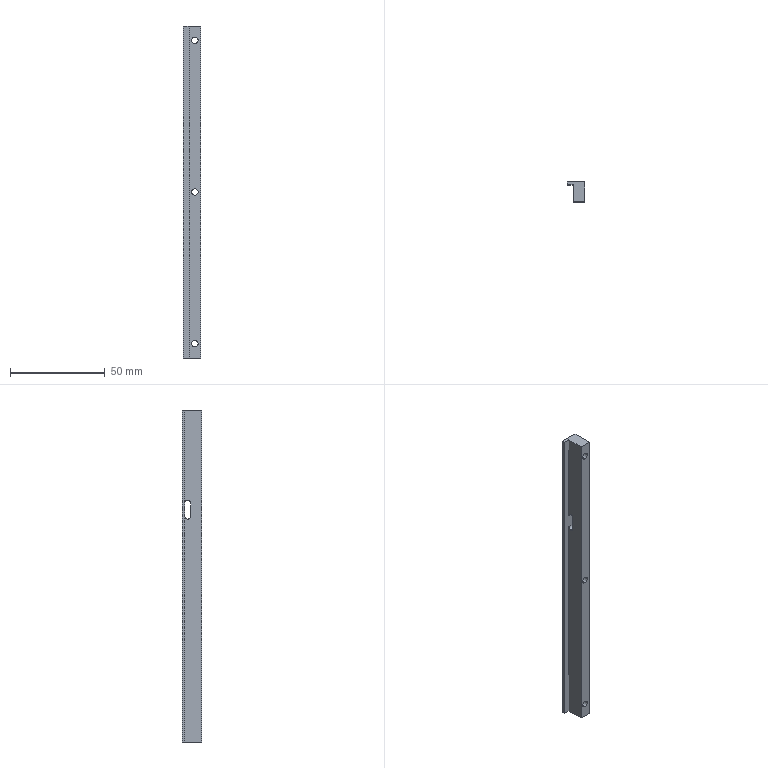Part | STEP file | PN_0006 | 1 solid | 19 faces | box 9 x 10.5 x 175 mm | volume 11358 mm3 | cylinder 10 | plane 9 | commonest cylinder face diameters 3.4 x6 3 x4
STEP:
#1=CARTESIAN_POINT('',(0.,0.,0.));
#2=DIRECTION('',(0.,0.,1.));
#3=DIRECTION('',(1.,0.,0.));
#4=AXIS2_PLACEMENT_3D('',#1,#2,#3);
#5=CARTESIAN_POINT('',(1.5,0.,-78.3));
#6=VERTEX_POINT('',#5);
#7=CARTESIAN_POINT('',(1.5,10.5,-78.3));
#8=VERTEX_POINT('',#7);
#9=CARTESIAN_POINT('',(1.5,10.5,-78.3));
#10=DIRECTION('',(0.,1.,0.));
#11=VECTOR('',#10,1.);
#12=LINE('',#9,#11);
#13=CARTESIAN_POINT('',(1.5,10.5,-80.));
#14=DIRECTION('',(0.,1.,0.));
#15=DIRECTION('',(0.,0.,1.));
#16=AXIS2_PLACEMENT_3D('',#13,#14,#15);
#17=CYLINDRICAL_SURFACE('',#16,1.7);
#18=CARTESIAN_POINT('',(6.283,0.));
#19=DIRECTION('',(0.,1.));
#20=VECTOR('',#19,1.);
#21=LINE('',#18,#20);
#22=(GEOMETRIC_REPRESENTATION_CONTEXT(2)PARAMETRIC_REPRESENTATION_CONTEXT()REPRESENTATION_CONTEXT('',''));
#23=DEFINITIONAL_REPRESENTATION('',(#21),#22);
#24=PCURVE('',#17,#23);
#25=CARTESIAN_POINT('',(1.5,10.5,-80.));
#26=DIRECTION('',(0.,1.,0.));
#27=DIRECTION('',(0.,0.,1.));
#28=AXIS2_PLACEMENT_3D('',#25,#26,#27);
#29=CYLINDRICAL_SURFACE('',#28,1.7);
#30=CARTESIAN_POINT('',(0.,0.));
#31=DIRECTION('',(0.,1.));
#32=VECTOR('',#31,1.);
#33=LINE('',#30,#32);
#34=(GEOMETRIC_REPRESENTATION_CONTEXT(2)PARAMETRIC_REPRESENTATION_CONTEXT()REPRESENTATION_CONTEXT('',''));
#35=DEFINITIONAL_REPRESENTATION('',(#33),#34);
#36=PCURVE('',#29,#35);
#37=SURFACE_CURVE('',#12,(#24,#36),.PCURVE_S1.);
#38=EDGE_CURVE('',#6,#8,#37,.T.);
#39=ORIENTED_EDGE('',*,*,#38,.T.);
#40=CARTESIAN_POINT('',(1.5,10.5,-81.7));
#41=VERTEX_POINT('',#40);
#42=CARTESIAN_POINT('',(1.5,10.5,-80.));
#43=DIRECTION('',(0.,1.,0.));
#44=DIRECTION('',(0.,0.,1.));
#45=AXIS2_PLACEMENT_3D('',#42,#43,#44);
#46=CIRCLE('',#45,1.7);
#47=CARTESIAN_POINT('',(0.,0.));
#48=DIRECTION('',(1.,0.));
#49=VECTOR('',#48,1.);
#50=LINE('',#47,#49);
#51=(GEOMETRIC_REPRESENTATION_CONTEXT(2)PARAMETRIC_REPRESENTATION_CONTEXT()REPRESENTATION_CONTEXT('',''));
#52=DEFINITIONAL_REPRESENTATION('',(#50),#51);
#53=PCURVE('',#17,#52);
#54=CARTESIAN_POINT('',(0.,10.5,0.));
#55=DIRECTION('',(0.,1.,0.));
#56=DIRECTION('',(0.,0.,1.));
#57=AXIS2_PLACEMENT_3D('',#54,#55,#56);
#58=PLANE('',#57);
#59=CARTESIAN_POINT('',(-80.,1.5));
#60=DIRECTION('',(1.,0.));
#61=AXIS2_PLACEMENT_2D('',#59,#60);
#62=CIRCLE('',#61,1.7);
#63=(GEOMETRIC_REPRESENTATION_CONTEXT(2)PARAMETRIC_REPRESENTATION_CONTEXT()REPRESENTATION_CONTEXT('',''));
#64=DEFINITIONAL_REPRESENTATION('',(#62),#63);
#65=PCURVE('',#58,#64);
#66=SURFACE_CURVE('',#46,(#53,#65),.PCURVE_S1.);
#67=EDGE_CURVE('',#41,#8,#66,.T.);
#68=ORIENTED_EDGE('',*,*,#67,.F.);
#69=CARTESIAN_POINT('',(1.5,0.,-81.7));
#70=VERTEX_POINT('',#69);
#71=CARTESIAN_POINT('',(1.5,10.5,-81.7));
#72=DIRECTION('',(0.,1.,0.));
#73=VECTOR('',#72,1.);
#74=LINE('',#71,#73);
#75=CARTESIAN_POINT('',(3.142,0.));
#76=DIRECTION('',(0.,1.));
#77=VECTOR('',#76,1.);
#78=LINE('',#75,#77);
#79=(GEOMETRIC_REPRESENTATION_CONTEXT(2)PARAMETRIC_REPRESENTATION_CONTEXT()REPRESENTATION_CONTEXT('',''));
#80=DEFINITIONAL_REPRESENTATION('',(#78),#79);
#81=PCURVE('',#17,#80);
#82=CARTESIAN_POINT('',(3.142,0.));
#83=DIRECTION('',(0.,1.));
#84=VECTOR('',#83,1.);
#85=LINE('',#82,#84);
#86=(GEOMETRIC_REPRESENTATION_CONTEXT(2)PARAMETRIC_REPRESENTATION_CONTEXT()REPRESENTATION_CONTEXT('',''));
#87=DEFINITIONAL_REPRESENTATION('',(#85),#86);
#88=PCURVE('',#29,#87);
#89=SURFACE_CURVE('',#74,(#81,#88),.PCURVE_S1.);
#90=EDGE_CURVE('',#70,#41,#89,.T.);
#91=ORIENTED_EDGE('',*,*,#90,.F.);
#92=CARTESIAN_POINT('',(1.5,0.,-80.));
#93=DIRECTION('',(0.,1.,0.));
#94=DIRECTION('',(0.,0.,1.));
#95=AXIS2_PLACEMENT_3D('',#92,#93,#94);
#96=CIRCLE('',#95,1.7);
#97=CARTESIAN_POINT('',(0.,-10.5));
#98=DIRECTION('',(1.,0.));
#99=VECTOR('',#98,1.);
#100=LINE('',#97,#99);
#101=(GEOMETRIC_REPRESENTATION_CONTEXT(2)PARAMETRIC_REPRESENTATION_CONTEXT()REPRESENTATION_CONTEXT('',''));
#102=DEFINITIONAL_REPRESENTATION('',(#100),#101);
#103=PCURVE('',#17,#102);
#104=CARTESIAN_POINT('',(0.,0.,0.));
#105=DIRECTION('',(0.,1.,0.));
#106=DIRECTION('',(0.,0.,1.));
#107=AXIS2_PLACEMENT_3D('',#104,#105,#106);
#108=PLANE('',#107);
#109=CARTESIAN_POINT('',(-80.,1.5));
#110=DIRECTION('',(1.,0.));
#111=AXIS2_PLACEMENT_2D('',#109,#110);
#112=CIRCLE('',#111,1.7);
#113=(GEOMETRIC_REPRESENTATION_CONTEXT(2)PARAMETRIC_REPRESENTATION_CONTEXT()REPRESENTATION_CONTEXT('',''));
#114=DEFINITIONAL_REPRESENTATION('',(#112),#113);
#115=PCURVE('',#108,#114);
#116=SURFACE_CURVE('',#96,(#103,#115),.PCURVE_S1.);
#117=EDGE_CURVE('',#70,#6,#116,.T.);
#118=ORIENTED_EDGE('',*,*,#117,.T.);
#119=EDGE_LOOP('',(#39,#68,#91,#118));
#120=FACE_BOUND('',#119,.F.);
#121=ADVANCED_FACE('',(#120),#17,.F.);
#122=CARTESIAN_POINT('',(1.5,0.,1.7));
#123=VERTEX_POINT('',#122);
#124=CARTESIAN_POINT('',(1.5,10.5,1.7));
#125=VERTEX_POINT('',#124);
#126=CARTESIAN_POINT('',(1.5,10.5,1.7));
#127=DIRECTION('',(0.,1.,0.));
#128=VECTOR('',#127,1.);
#129=LINE('',#126,#128);
#130=CARTESIAN_POINT('',(1.5,10.5,0.));
#131=DIRECTION('',(0.,1.,0.));
#132=DIRECTION('',(0.,0.,1.));
#133=AXIS2_PLACEMENT_3D('',#130,#131,#132);
#134=CYLINDRICAL_SURFACE('',#133,1.7);
#135=CARTESIAN_POINT('',(6.283,0.));
#136=DIRECTION('',(0.,1.));
#137=VECTOR('',#136,1.);
#138=LINE('',#135,#137);
#139=(GEOMETRIC_REPRESENTATION_CONTEXT(2)PARAMETRIC_REPRESENTATION_CONTEXT()REPRESENTATION_CONTEXT('',''));
#140=DEFINITIONAL_REPRESENTATION('',(#138),#139);
#141=PCURVE('',#134,#140);
#142=CARTESIAN_POINT('',(1.5,10.5,0.));
#143=DIRECTION('',(0.,1.,0.));
#144=DIRECTION('',(0.,0.,1.));
#145=AXIS2_PLACEMENT_3D('',#142,#143,#144);
#146=CYLINDRICAL_SURFACE('',#145,1.7);
#147=CARTESIAN_POINT('',(0.,0.));
#148=DIRECTION('',(0.,1.));
#149=VECTOR('',#148,1.);
#150=LINE('',#147,#149);
#151=(GEOMETRIC_REPRESENTATION_CONTEXT(2)PARAMETRIC_REPRESENTATION_CONTEXT()REPRESENTATION_CONTEXT('',''));
#152=DEFINITIONAL_REPRESENTATION('',(#150),#151);
#153=PCURVE('',#146,#152);
#154=SURFACE_CURVE('',#129,(#141,#153),.PCURVE_S1.);
#155=EDGE_CURVE('',#123,#125,#154,.T.);
#156=ORIENTED_EDGE('',*,*,#155,.T.);
#157=CARTESIAN_POINT('',(1.5,10.5,-1.7));
#158=VERTEX_POINT('',#157);
#159=CARTESIAN_POINT('',(1.5,10.5,0.));
#160=DIRECTION('',(0.,1.,0.));
#161=DIRECTION('',(0.,0.,1.));
#162=AXIS2_PLACEMENT_3D('',#159,#160,#161);
#163=CIRCLE('',#162,1.7);
#164=CARTESIAN_POINT('',(0.,0.));
#165=DIRECTION('',(1.,0.));
#166=VECTOR('',#165,1.);
#167=LINE('',#164,#166);
#168=(GEOMETRIC_REPRESENTATION_CONTEXT(2)PARAMETRIC_REPRESENTATION_CONTEXT()REPRESENTATION_CONTEXT('',''));
#169=DEFINITIONAL_REPRESENTATION('',(#167),#168);
#170=PCURVE('',#134,#169);
#171=CARTESIAN_POINT('',(0.,1.5));
#172=DIRECTION('',(1.,0.));
#173=AXIS2_PLACEMENT_2D('',#171,#172);
#174=CIRCLE('',#173,1.7);
#175=(GEOMETRIC_REPRESENTATION_CONTEXT(2)PARAMETRIC_REPRESENTATION_CONTEXT()REPRESENTATION_CONTEXT('',''));
#176=DEFINITIONAL_REPRESENTATION('',(#174),#175);
#177=PCURVE('',#58,#176);
#178=SURFACE_CURVE('',#163,(#170,#177),.PCURVE_S1.);
#179=EDGE_CURVE('',#158,#125,#178,.T.);
#180=ORIENTED_EDGE('',*,*,#179,.F.);
#181=CARTESIAN_POINT('',(1.5,0.,-1.7));
#182=VERTEX_POINT('',#181);
#183=CARTESIAN_POINT('',(1.5,10.5,-1.7));
#184=DIRECTION('',(0.,1.,0.));
#185=VECTOR('',#184,1.);
#186=LINE('',#183,#185);
#187=CARTESIAN_POINT('',(3.142,0.));
#188=DIRECTION('',(0.,1.));
#189=VECTOR('',#188,1.);
#190=LINE('',#187,#189);
#191=(GEOMETRIC_REPRESENTATION_CONTEXT(2)PARAMETRIC_REPRESENTATION_CONTEXT()REPRESENTATION_CONTEXT('',''));
#192=DEFINITIONAL_REPRESENTATION('',(#190),#191);
#193=PCURVE('',#134,#192);
#194=CARTESIAN_POINT('',(3.142,0.));
#195=DIRECTION('',(0.,1.));
#196=VECTOR('',#195,1.);
#197=LINE('',#194,#196);
#198=(GEOMETRIC_REPRESENTATION_CONTEXT(2)PARAMETRIC_REPRESENTATION_CONTEXT()REPRESENTATION_CONTEXT('',''));
#199=DEFINITIONAL_REPRESENTATION('',(#197),#198);
#200=PCURVE('',#146,#199);
#201=SURFACE_CURVE('',#186,(#193,#200),.PCURVE_S1.);
#202=EDGE_CURVE('',#182,#158,#201,.T.);
#203=ORIENTED_EDGE('',*,*,#202,.F.);
#204=CARTESIAN_POINT('',(1.5,0.,0.));
#205=DIRECTION('',(0.,1.,0.));
#206=DIRECTION('',(0.,0.,1.));
#207=AXIS2_PLACEMENT_3D('',#204,#205,#206);
#208=CIRCLE('',#207,1.7);
#209=CARTESIAN_POINT('',(0.,-10.5));
#210=DIRECTION('',(1.,0.));
#211=VECTOR('',#210,1.);
#212=LINE('',#209,#211);
#213=(GEOMETRIC_REPRESENTATION_CONTEXT(2)PARAMETRIC_REPRESENTATION_CONTEXT()REPRESENTATION_CONTEXT('',''));
#214=DEFINITIONAL_REPRESENTATION('',(#212),#213);
#215=PCURVE('',#134,#214);
#216=CARTESIAN_POINT('',(0.,1.5));
#217=DIRECTION('',(1.,0.));
#218=AXIS2_PLACEMENT_2D('',#216,#217);
#219=CIRCLE('',#218,1.7);
#220=(GEOMETRIC_REPRESENTATION_CONTEXT(2)PARAMETRIC_REPRESENTATION_CONTEXT()REPRESENTATION_CONTEXT('',''));
#221=DEFINITIONAL_REPRESENTATION('',(#219),#220);
#222=PCURVE('',#108,#221);
#223=SURFACE_CURVE('',#208,(#215,#222),.PCURVE_S1.);
#224=EDGE_CURVE('',#182,#123,#223,.T.);
#225=ORIENTED_EDGE('',*,*,#224,.T.);
#226=EDGE_LOOP('',(#156,#180,#203,#225));
#227=FACE_BOUND('',#226,.F.);
#228=ADVANCED_FACE('',(#227),#134,.F.);
#229=CARTESIAN_POINT('',(1.5,0.,81.7));
#230=VERTEX_POINT('',#229);
#231=CARTESIAN_POINT('',(1.5,10.5,81.7));
#232=VERTEX_POINT('',#231);
#233=CARTESIAN_POINT('',(1.5,10.5,81.7));
#234=DIRECTION('',(0.,1.,0.));
#235=VECTOR('',#234,1.);
#236=LINE('',#233,#235);
#237=CARTESIAN_POINT('',(1.5,10.5,80.));
#238=DIRECTION('',(0.,1.,0.));
#239=DIRECTION('',(0.,0.,1.));
#240=AXIS2_PLACEMENT_3D('',#237,#238,#239);
#241=CYLINDRICAL_SURFACE('',#240,1.7);
#242=CARTESIAN_POINT('',(6.283,0.));
#243=DIRECTION('',(0.,1.));
#244=VECTOR('',#243,1.);
#245=LINE('',#242,#244);
#246=(GEOMETRIC_REPRESENTATION_CONTEXT(2)PARAMETRIC_REPRESENTATION_CONTEXT()REPRESENTATION_CONTEXT('',''));
#247=DEFINITIONAL_REPRESENTATION('',(#245),#246);
#248=PCURVE('',#241,#247);
#249=CARTESIAN_POINT('',(1.5,10.5,80.));
#250=DIRECTION('',(0.,1.,0.));
#251=DIRECTION('',(0.,0.,1.));
#252=AXIS2_PLACEMENT_3D('',#249,#250,#251);
#253=CYLINDRICAL_SURFACE('',#252,1.7);
#254=CARTESIAN_POINT('',(0.,0.));
#255=DIRECTION('',(0.,1.));
#256=VECTOR('',#255,1.);
#257=LINE('',#254,#256);
#258=(GEOMETRIC_REPRESENTATION_CONTEXT(2)PARAMETRIC_REPRESENTATION_CONTEXT()REPRESENTATION_CONTEXT('',''));
#259=DEFINITIONAL_REPRESENTATION('',(#257),#258);
#260=PCURVE('',#253,#259);
#261=SURFACE_CURVE('',#236,(#248,#260),.PCURVE_S1.);
#262=EDGE_CURVE('',#230,#232,#261,.T.);
#263=ORIENTED_EDGE('',*,*,#262,.T.);
#264=CARTESIAN_POINT('',(1.5,10.5,78.3));
#265=VERTEX_POINT('',#264);
#266=CARTESIAN_POINT('',(1.5,10.5,80.));
#267=DIRECTION('',(0.,1.,0.));
#268=DIRECTION('',(0.,0.,1.));
#269=AXIS2_PLACEMENT_3D('',#266,#267,#268);
#270=CIRCLE('',#269,1.7);
#271=CARTESIAN_POINT('',(0.,0.));
#272=DIRECTION('',(1.,0.));
#273=VECTOR('',#272,1.);
#274=LINE('',#271,#273);
#275=(GEOMETRIC_REPRESENTATION_CONTEXT(2)PARAMETRIC_REPRESENTATION_CONTEXT()REPRESENTATION_CONTEXT('',''));
#276=DEFINITIONAL_REPRESENTATION('',(#274),#275);
#277=PCURVE('',#241,#276);
#278=CARTESIAN_POINT('',(80.,1.5));
#279=DIRECTION('',(1.,0.));
#280=AXIS2_PLACEMENT_2D('',#278,#279);
#281=CIRCLE('',#280,1.7);
#282=(GEOMETRIC_REPRESENTATION_CONTEXT(2)PARAMETRIC_REPRESENTATION_CONTEXT()REPRESENTATION_CONTEXT('',''));
#283=DEFINITIONAL_REPRESENTATION('',(#281),#282);
#284=PCURVE('',#58,#283);
#285=SURFACE_CURVE('',#270,(#277,#284),.PCURVE_S1.);
#286=EDGE_CURVE('',#265,#232,#285,.T.);
#287=ORIENTED_EDGE('',*,*,#286,.F.);
#288=CARTESIAN_POINT('',(1.5,0.,78.3));
#289=VERTEX_POINT('',#288);
#290=CARTESIAN_POINT('',(1.5,10.5,78.3));
#291=DIRECTION('',(0.,1.,0.));
#292=VECTOR('',#291,1.);
#293=LINE('',#290,#292);
#294=CARTESIAN_POINT('',(3.142,0.));
#295=DIRECTION('',(0.,1.));
#296=VECTOR('',#295,1.);
#297=LINE('',#294,#296);
#298=(GEOMETRIC_REPRESENTATION_CONTEXT(2)PARAMETRIC_REPRESENTATION_CONTEXT()REPRESENTATION_CONTEXT('',''));
#299=DEFINITIONAL_REPRESENTATION('',(#297),#298);
#300=PCURVE('',#241,#299);
#301=CARTESIAN_POINT('',(3.142,0.));
#302=DIRECTION('',(0.,1.));
#303=VECTOR('',#302,1.);
#304=LINE('',#301,#303);
#305=(GEOMETRIC_REPRESENTATION_CONTEXT(2)PARAMETRIC_REPRESENTATION_CONTEXT()REPRESENTATION_CONTEXT('',''));
#306=DEFINITIONAL_REPRESENTATION('',(#304),#305);
#307=PCURVE('',#253,#306);
#308=SURFACE_CURVE('',#293,(#300,#307),.PCURVE_S1.);
#309=EDGE_CURVE('',#289,#265,#308,.T.);
#310=ORIENTED_EDGE('',*,*,#309,.F.);
#311=CARTESIAN_POINT('',(1.5,0.,80.));
#312=DIRECTION('',(0.,1.,0.));
#313=DIRECTION('',(0.,0.,1.));
#314=AXIS2_PLACEMENT_3D('',#311,#312,#313);
#315=CIRCLE('',#314,1.7);
#316=CARTESIAN_POINT('',(0.,-10.5));
#317=DIRECTION('',(1.,0.));
#318=VECTOR('',#317,1.);
#319=LINE('',#316,#318);
#320=(GEOMETRIC_REPRESENTATION_CONTEXT(2)PARAMETRIC_REPRESENTATION_CONTEXT()REPRESENTATION_CONTEXT('',''));
#321=DEFINITIONAL_REPRESENTATION('',(#319),#320);
#322=PCURVE('',#241,#321);
#323=CARTESIAN_POINT('',(80.,1.5));
#324=DIRECTION('',(1.,0.));
#325=AXIS2_PLACEMENT_2D('',#323,#324);
#326=CIRCLE('',#325,1.7);
#327=(GEOMETRIC_REPRESENTATION_CONTEXT(2)PARAMETRIC_REPRESENTATION_CONTEXT()REPRESENTATION_CONTEXT('',''));
#328=DEFINITIONAL_REPRESENTATION('',(#326),#327);
#329=PCURVE('',#108,#328);
#330=SURFACE_CURVE('',#315,(#322,#329),.PCURVE_S1.);
#331=EDGE_CURVE('',#289,#230,#330,.T.);
#332=ORIENTED_EDGE('',*,*,#331,.T.);
#333=EDGE_LOOP('',(#263,#287,#310,#332));
#334=FACE_BOUND('',#333,.F.);
#335=ADVANCED_FACE('',(#334),#241,.F.);
#336=CARTESIAN_POINT('',(4.5,6.,38.5));
#337=VERTEX_POINT('',#336);
#338=CARTESIAN_POINT('',(4.5,7.5,40.));
#339=VERTEX_POINT('',#338);
#340=CARTESIAN_POINT('',(4.5,7.5,38.5));
#341=DIRECTION('',(-1.,0.,0.));
#342=DIRECTION('',(0.,0.,1.));
#343=AXIS2_PLACEMENT_3D('',#340,#341,#342);
#344=CIRCLE('',#343,1.5);
#345=CARTESIAN_POINT('',(4.5,10.5,-87.5));
#346=DIRECTION('',(-1.,0.,0.));
#347=DIRECTION('',(0.,0.,1.));
#348=AXIS2_PLACEMENT_3D('',#345,#346,#347);
#349=PLANE('',#348);
#350=CARTESIAN_POINT('',(126.,-3.));
#351=DIRECTION('',(1.,0.));
#352=AXIS2_PLACEMENT_2D('',#350,#351);
#353=CIRCLE('',#352,1.5);
#354=(GEOMETRIC_REPRESENTATION_CONTEXT(2)PARAMETRIC_REPRESENTATION_CONTEXT()REPRESENTATION_CONTEXT('',''));
#355=DEFINITIONAL_REPRESENTATION('',(#353),#354);
#356=PCURVE('',#349,#355);
#357=CARTESIAN_POINT('',(4.5,7.5,38.5));
#358=DIRECTION('',(1.,0.,0.));
#359=DIRECTION('',(0.,0.,-1.));
#360=AXIS2_PLACEMENT_3D('',#357,#358,#359);
#361=CYLINDRICAL_SURFACE('',#360,1.5);
#362=CARTESIAN_POINT('',(9.425,0.));
#363=DIRECTION('',(-1.,0.));
#364=VECTOR('',#363,1.);
#365=LINE('',#362,#364);
#366=(GEOMETRIC_REPRESENTATION_CONTEXT(2)PARAMETRIC_REPRESENTATION_CONTEXT()REPRESENTATION_CONTEXT('',''));
#367=DEFINITIONAL_REPRESENTATION('',(#365),#366);
#368=PCURVE('',#361,#367);
#369=SURFACE_CURVE('',#344,(#356,#368),.PCURVE_S1.);
#370=EDGE_CURVE('',#337,#339,#369,.T.);
#371=ORIENTED_EDGE('',*,*,#370,.T.);
#372=CARTESIAN_POINT('',(4.5,9.,38.5));
#373=VERTEX_POINT('',#372);
#374=CARTESIAN_POINT('',(4.5,7.5,38.5));
#375=DIRECTION('',(-1.,0.,0.));
#376=DIRECTION('',(0.,0.,1.));
#377=AXIS2_PLACEMENT_3D('',#374,#375,#376);
#378=CIRCLE('',#377,1.5);
#379=CARTESIAN_POINT('',(126.,-3.));
#380=DIRECTION('',(1.,0.));
#381=AXIS2_PLACEMENT_2D('',#379,#380);
#382=CIRCLE('',#381,1.5);
#383=(GEOMETRIC_REPRESENTATION_CONTEXT(2)PARAMETRIC_REPRESENTATION_CONTEXT()REPRESENTATION_CONTEXT('',''));
#384=DEFINITIONAL_REPRESENTATION('',(#382),#383);
#385=PCURVE('',#349,#384);
#386=CARTESIAN_POINT('',(-4.5,7.5,38.5));
#387=DIRECTION('',(1.,0.,0.));
#388=DIRECTION('',(0.,0.,-1.));
#389=AXIS2_PLACEMENT_3D('',#386,#387,#388);
#390=CYLINDRICAL_SURFACE('',#389,1.5);
#391=CARTESIAN_POINT('',(3.142,9.));
#392=DIRECTION('',(-1.,0.));
#393=VECTOR('',#392,1.);
#394=LINE('',#391,#393);
#395=(GEOMETRIC_REPRESENTATION_CONTEXT(2)PARAMETRIC_REPRESENTATION_CONTEXT()REPRESENTATION_CONTEXT('',''));
#396=DEFINITIONAL_REPRESENTATION('',(#394),#395);
#397=PCURVE('',#390,#396);
#398=SURFACE_CURVE('',#378,(#385,#397),.PCURVE_S1.);
#399=EDGE_CURVE('',#339,#373,#398,.T.);
#400=ORIENTED_EDGE('',*,*,#399,.T.);
#401=CARTESIAN_POINT('',(4.5,9.,31.5));
#402=VERTEX_POINT('',#401);
#403=CARTESIAN_POINT('',(4.5,9.,30.));
#404=DIRECTION('',(0.,0.,-1.));
#405=VECTOR('',#404,1.);
#406=LINE('',#403,#405);
#407=CARTESIAN_POINT('',(117.5,-1.5));
#408=DIRECTION('',(-1.,0.));
#409=VECTOR('',#408,1.);
#410=LINE('',#407,#409);
#411=(GEOMETRIC_REPRESENTATION_CONTEXT(2)PARAMETRIC_REPRESENTATION_CONTEXT()REPRESENTATION_CONTEXT('',''));
#412=DEFINITIONAL_REPRESENTATION('',(#410),#411);
#413=PCURVE('',#349,#412);
#414=CARTESIAN_POINT('',(-4.5,9.,-87.5));
#415=DIRECTION('',(0.,1.,0.));
#416=DIRECTION('',(0.,0.,1.));
#417=AXIS2_PLACEMENT_3D('',#414,#415,#416);
#418=PLANE('',#417);
#419=CARTESIAN_POINT('',(117.5,9.));
#420=DIRECTION('',(-1.,0.));
#421=VECTOR('',#420,1.);
#422=LINE('',#419,#421);
#423=(GEOMETRIC_REPRESENTATION_CONTEXT(2)PARAMETRIC_REPRESENTATION_CONTEXT()REPRESENTATION_CONTEXT('',''));
#424=DEFINITIONAL_REPRESENTATION('',(#422),#423);
#425=PCURVE('',#418,#424);
#426=SURFACE_CURVE('',#406,(#413,#425),.PCURVE_S1.);
#427=EDGE_CURVE('',#373,#402,#426,.T.);
#428=ORIENTED_EDGE('',*,*,#427,.T.);
#429=CARTESIAN_POINT('',(4.5,7.5,30.));
#430=VERTEX_POINT('',#429);
#431=CARTESIAN_POINT('',(4.5,7.5,31.5));
#432=DIRECTION('',(-1.,0.,0.));
#433=DIRECTION('',(0.,0.,1.));
#434=AXIS2_PLACEMENT_3D('',#431,#432,#433);
#435=CIRCLE('',#434,1.5);
#436=CARTESIAN_POINT('',(119.,-3.));
#437=DIRECTION('',(1.,0.));
#438=AXIS2_PLACEMENT_2D('',#436,#437);
#439=CIRCLE('',#438,1.5);
#440=(GEOMETRIC_REPRESENTATION_CONTEXT(2)PARAMETRIC_REPRESENTATION_CONTEXT()REPRESENTATION_CONTEXT('',''));
#441=DEFINITIONAL_REPRESENTATION('',(#439),#440);
#442=PCURVE('',#349,#441);
#443=CARTESIAN_POINT('',(4.5,7.5,31.5));
#444=DIRECTION('',(1.,0.,0.));
#445=DIRECTION('',(0.,0.,-1.));
#446=AXIS2_PLACEMENT_3D('',#443,#444,#445);
#447=CYLINDRICAL_SURFACE('',#446,1.5);
#448=CARTESIAN_POINT('',(3.142,0.));
#449=DIRECTION('',(-1.,0.));
#450=VECTOR('',#449,1.);
#451=LINE('',#448,#450);
#452=(GEOMETRIC_REPRESENTATION_CONTEXT(2)PARAMETRIC_REPRESENTATION_CONTEXT()REPRESENTATION_CONTEXT('',''));
#453=DEFINITIONAL_REPRESENTATION('',(#451),#452);
#454=PCURVE('',#447,#453);
#455=SURFACE_CURVE('',#435,(#442,#454),.PCURVE_S1.);
#456=EDGE_CURVE('',#402,#430,#455,.T.);
#457=ORIENTED_EDGE('',*,*,#456,.T.);
#458=CARTESIAN_POINT('',(4.5,6.,31.5));
#459=VERTEX_POINT('',#458);
#460=CARTESIAN_POINT('',(4.5,7.5,31.5));
#461=DIRECTION('',(-1.,0.,0.));
#462=DIRECTION('',(0.,0.,1.));
#463=AXIS2_PLACEMENT_3D('',#460,#461,#462);
#464=CIRCLE('',#463,1.5);
#465=CARTESIAN_POINT('',(119.,-3.));
#466=DIRECTION('',(1.,0.));
#467=AXIS2_PLACEMENT_2D('',#465,#466);
#468=CIRCLE('',#467,1.5);
#469=(GEOMETRIC_REPRESENTATION_CONTEXT(2)PARAMETRIC_REPRESENTATION_CONTEXT()REPRESENTATION_CONTEXT('',''));
#470=DEFINITIONAL_REPRESENTATION('',(#468),#469);
#471=PCURVE('',#349,#470);
#472=CARTESIAN_POINT('',(4.5,7.5,31.5));
#473=DIRECTION('',(1.,0.,0.));
#474=DIRECTION('',(0.,0.,-1.));
#475=AXIS2_PLACEMENT_3D('',#472,#473,#474);
#476=CYLINDRICAL_SURFACE('',#475,1.5);
#477=CARTESIAN_POINT('',(9.425,0.));
#478=DIRECTION('',(-1.,0.));
#479=VECTOR('',#478,1.);
#480=LINE('',#477,#479);
#481=(GEOMETRIC_REPRESENTATION_CONTEXT(2)PARAMETRIC_REPRESENTATION_CONTEXT()REPRESENTATION_CONTEXT('',''));
#482=DEFINITIONAL_REPRESENTATION('',(#480),#481);
#483=PCURVE('',#476,#482);
#484=SURFACE_CURVE('',#464,(#471,#483),.PCURVE_S1.);
#485=EDGE_CURVE('',#430,#459,#484,.T.);
#486=ORIENTED_EDGE('',*,*,#485,.T.);
#487=CARTESIAN_POINT('',(4.5,6.,30.));
#488=DIRECTION('',(0.,0.,1.));
#489=VECTOR('',#488,1.);
#490=LINE('',#487,#489);
#491=CARTESIAN_POINT('',(117.5,-4.5));
#492=DIRECTION('',(1.,0.));
#493=VECTOR('',#492,1.);
#494=LINE('',#491,#493);
#495=(GEOMETRIC_REPRESENTATION_CONTEXT(2)PARAMETRIC_REPRESENTATION_CONTEXT()REPRESENTATION_CONTEXT('',''));
#496=DEFINITIONAL_REPRESENTATION('',(#494),#495);
#497=PCURVE('',#349,#496);
#498=CARTESIAN_POINT('',(4.5,6.,30.));
#499=DIRECTION('',(0.,-1.,0.));
#500=DIRECTION('',(0.,0.,-1.));
#501=AXIS2_PLACEMENT_3D('',#498,#499,#500);
#502=PLANE('',#501);
#503=CARTESIAN_POINT('',(0.,0.));
#504=DIRECTION('',(-1.,0.));
#505=VECTOR('',#504,1.);
#506=LINE('',#503,#505);
#507=(GEOMETRIC_REPRESENTATION_CONTEXT(2)PARAMETRIC_REPRESENTATION_CONTEXT()REPRESENTATION_CONTEXT('',''));
#508=DEFINITIONAL_REPRESENTATION('',(#506),#507);
#509=PCURVE('',#502,#508);
#510=SURFACE_CURVE('',#490,(#497,#509),.PCURVE_S1.);
#511=EDGE_CURVE('',#459,#337,#510,.T.);
#512=ORIENTED_EDGE('',*,*,#511,.T.);
#513=EDGE_LOOP('',(#371,#400,#428,#457,#486,#512));
#514=FACE_BOUND('',#513,.T.);
#515=CARTESIAN_POINT('',(4.5,0.,87.5));
#516=VERTEX_POINT('',#515);
#517=CARTESIAN_POINT('',(4.5,0.,-87.5));
#518=VERTEX_POINT('',#517);
#519=CARTESIAN_POINT('',(4.5,0.,-87.5));
#520=DIRECTION('',(0.,0.,-1.));
#521=VECTOR('',#520,1.);
#522=LINE('',#519,#521);
#523=CARTESIAN_POINT('',(0.,-10.5));
#524=DIRECTION('',(-1.,0.));
#525=VECTOR('',#524,1.);
#526=LINE('',#523,#525);
#527=(GEOMETRIC_REPRESENTATION_CONTEXT(2)PARAMETRIC_REPRESENTATION_CONTEXT()REPRESENTATION_CONTEXT('',''));
#528=DEFINITIONAL_REPRESENTATION('',(#526),#527);
#529=PCURVE('',#349,#528);
#530=CARTESIAN_POINT('',(-87.5,4.5));
#531=DIRECTION('',(-1.,0.));
#532=VECTOR('',#531,1.);
#533=LINE('',#530,#532);
#534=(GEOMETRIC_REPRESENTATION_CONTEXT(2)PARAMETRIC_REPRESENTATION_CONTEXT()REPRESENTATION_CONTEXT('',''));
#535=DEFINITIONAL_REPRESENTATION('',(#533),#534);
#536=PCURVE('',#108,#535);
#537=SURFACE_CURVE('',#522,(#529,#536),.PCURVE_S1.);
#538=EDGE_CURVE('',#516,#518,#537,.T.);
#539=ORIENTED_EDGE('',*,*,#538,.T.);
#540=CARTESIAN_POINT('',(4.5,10.5,-87.5));
#541=VERTEX_POINT('',#540);
#542=CARTESIAN_POINT('',(4.5,10.5,-87.5));
#543=DIRECTION('',(0.,-1.,0.));
#544=VECTOR('',#543,1.);
#545=LINE('',#542,#544);
#546=CARTESIAN_POINT('',(0.,0.));
#547=DIRECTION('',(0.,-1.));
#548=VECTOR('',#547,1.);
#549=LINE('',#546,#548);
#550=(GEOMETRIC_REPRESENTATION_CONTEXT(2)PARAMETRIC_REPRESENTATION_CONTEXT()REPRESENTATION_CONTEXT('',''));
#551=DEFINITIONAL_REPRESENTATION('',(#549),#550);
#552=PCURVE('',#349,#551);
#553=CARTESIAN_POINT('',(-4.5,10.5,-87.5));
#554=DIRECTION('',(0.,0.,1.));
#555=DIRECTION('',(1.,0.,0.));
#556=AXIS2_PLACEMENT_3D('',#553,#554,#555);
#557=PLANE('',#556);
#558=CARTESIAN_POINT('',(9.,0.));
#559=DIRECTION('',(0.,-1.));
#560=VECTOR('',#559,1.);
#561=LINE('',#558,#560);
#562=(GEOMETRIC_REPRESENTATION_CONTEXT(2)PARAMETRIC_REPRESENTATION_CONTEXT()REPRESENTATION_CONTEXT('',''));
#563=DEFINITIONAL_REPRESENTATION('',(#561),#562);
#564=PCURVE('',#557,#563);
#565=SURFACE_CURVE('',#545,(#552,#564),.PCURVE_S1.);
#566=EDGE_CURVE('',#541,#518,#565,.T.);
#567=ORIENTED_EDGE('',*,*,#566,.F.);
#568=CARTESIAN_POINT('',(4.5,10.5,87.5));
#569=VERTEX_POINT('',#568);
#570=CARTESIAN_POINT('',(4.5,10.5,-87.5));
#571=DIRECTION('',(0.,0.,-1.));
#572=VECTOR('',#571,1.);
#573=LINE('',#570,#572);
#574=CARTESIAN_POINT('',(0.,0.));
#575=DIRECTION('',(-1.,0.));
#576=VECTOR('',#575,1.);
#577=LINE('',#574,#576);
#578=(GEOMETRIC_REPRESENTATION_CONTEXT(2)PARAMETRIC_REPRESENTATION_CONTEXT()REPRESENTATION_CONTEXT('',''));
#579=DEFINITIONAL_REPRESENTATION('',(#577),#578);
#580=PCURVE('',#349,#579);
#581=CARTESIAN_POINT('',(-87.5,4.5));
#582=DIRECTION('',(-1.,0.));
#583=VECTOR('',#582,1.);
#584=LINE('',#581,#583);
#585=(GEOMETRIC_REPRESENTATION_CONTEXT(2)PARAMETRIC_REPRESENTATION_CONTEXT()REPRESENTATION_CONTEXT('',''));
#586=DEFINITIONAL_REPRESENTATION('',(#584),#585);
#587=PCURVE('',#58,#586);
#588=SURFACE_CURVE('',#573,(#580,#587),.PCURVE_S1.);
#589=EDGE_CURVE('',#569,#541,#588,.T.);
#590=ORIENTED_EDGE('',*,*,#589,.F.);
#591=CARTESIAN_POINT('',(4.5,10.5,87.5));
#592=DIRECTION('',(0.,-1.,0.));
#593=VECTOR('',#592,1.);
#594=LINE('',#591,#593);
#595=CARTESIAN_POINT('',(175.,0.));
#596=DIRECTION('',(0.,-1.));
#597=VECTOR('',#596,1.);
#598=LINE('',#595,#597);
#599=(GEOMETRIC_REPRESENTATION_CONTEXT(2)PARAMETRIC_REPRESENTATION_CONTEXT()REPRESENTATION_CONTEXT('',''));
#600=DEFINITIONAL_REPRESENTATION('',(#598),#599);
#601=PCURVE('',#349,#600);
#602=CARTESIAN_POINT('',(-4.5,10.5,87.5));
#603=DIRECTION('',(0.,0.,-1.));
#604=DIRECTION('',(-1.,0.,0.));
#605=AXIS2_PLACEMENT_3D('',#602,#603,#604);
#606=PLANE('',#605);
#607=CARTESIAN_POINT('',(-9.,0.));
#608=DIRECTION('',(0.,-1.));
#609=VECTOR('',#608,1.);
#610=LINE('',#607,#609);
#611=(GEOMETRIC_REPRESENTATION_CONTEXT(2)PARAMETRIC_REPRESENTATION_CONTEXT()REPRESENTATION_CONTEXT('',''));
#612=DEFINITIONAL_REPRESENTATION('',(#610),#611);
#613=PCURVE('',#606,#612);
#614=SURFACE_CURVE('',#594,(#601,#613),.PCURVE_S1.);
#615=EDGE_CURVE('',#569,#516,#614,.T.);
#616=ORIENTED_EDGE('',*,*,#615,.T.);
#617=EDGE_LOOP('',(#539,#567,#590,#616));
#618=FACE_BOUND('',#617,.T.);
#619=ADVANCED_FACE('',(#514,#618),#349,.F.);
#620=CARTESIAN_POINT('',(-1.5,0.,-87.5));
#621=VERTEX_POINT('',#620);
#622=CARTESIAN_POINT('',(-1.5,9.,-87.5));
#623=VERTEX_POINT('',#622);
#624=CARTESIAN_POINT('',(-1.5,0.,-87.5));
#625=DIRECTION('',(0.,1.,0.));
#626=VECTOR('',#625,1.);
#627=LINE('',#624,#626);
#628=CARTESIAN_POINT('',(3.,-10.5));
#629=DIRECTION('',(0.,1.));
#630=VECTOR('',#629,1.);
#631=LINE('',#628,#630);
#632=(GEOMETRIC_REPRESENTATION_CONTEXT(2)PARAMETRIC_REPRESENTATION_CONTEXT()REPRESENTATION_CONTEXT('',''));
#633=DEFINITIONAL_REPRESENTATION('',(#631),#632);
#634=PCURVE('',#557,#633);
#635=CARTESIAN_POINT('',(-1.5,0.,-87.5));
#636=DIRECTION('',(1.,0.,0.));
#637=DIRECTION('',(0.,0.,-1.));
#638=AXIS2_PLACEMENT_3D('',#635,#636,#637);
#639=PLANE('',#638);
#640=CARTESIAN_POINT('',(0.,0.));
#641=DIRECTION('',(0.,1.));
#642=VECTOR('',#641,1.);
#643=LINE('',#640,#642);
#644=(GEOMETRIC_REPRESENTATION_CONTEXT(2)PARAMETRIC_REPRESENTATION_CONTEXT()REPRESENTATION_CONTEXT('',''));
#645=DEFINITIONAL_REPRESENTATION('',(#643),#644);
#646=PCURVE('',#639,#645);
#647=SURFACE_CURVE('',#627,(#634,#646),.PCURVE_S1.);
#648=EDGE_CURVE('',#621,#623,#647,.T.);
#649=ORIENTED_EDGE('',*,*,#648,.T.);
#650=CARTESIAN_POINT('',(-4.5,9.,-87.5));
#651=VERTEX_POINT('',#650);
#652=CARTESIAN_POINT('',(-4.5,9.,-87.5));
#653=DIRECTION('',(-1.,0.,0.));
#654=VECTOR('',#653,1.);
#655=LINE('',#652,#654);
#656=CARTESIAN_POINT('',(0.,-1.5));
#657=DIRECTION('',(-1.,0.));
#658=VECTOR('',#657,1.);
#659=LINE('',#656,#658);
#660=(GEOMETRIC_REPRESENTATION_CONTEXT(2)PARAMETRIC_REPRESENTATION_CONTEXT()REPRESENTATION_CONTEXT('',''));
#661=DEFINITIONAL_REPRESENTATION('',(#659),#660);
#662=PCURVE('',#557,#661);
#663=CARTESIAN_POINT('',(0.,0.));
#664=DIRECTION('',(0.,-1.));
#665=VECTOR('',#664,1.);
#666=LINE('',#663,#665);
#667=(GEOMETRIC_REPRESENTATION_CONTEXT(2)PARAMETRIC_REPRESENTATION_CONTEXT()REPRESENTATION_CONTEXT('',''));
#668=DEFINITIONAL_REPRESENTATION('',(#666),#667);
#669=PCURVE('',#418,#668);
#670=SURFACE_CURVE('',#655,(#662,#669),.PCURVE_S1.);
#671=EDGE_CURVE('',#623,#651,#670,.T.);
#672=ORIENTED_EDGE('',*,*,#671,.T.);
#673=CARTESIAN_POINT('',(-4.5,10.5,-87.5));
#674=VERTEX_POINT('',#673);
#675=CARTESIAN_POINT('',(-4.5,10.5,-87.5));
#676=DIRECTION('',(0.,-1.,0.));
#677=VECTOR('',#676,1.);
#678=LINE('',#675,#677);
#679=CARTESIAN_POINT('',(0.,0.));
#680=DIRECTION('',(0.,-1.));
#681=VECTOR('',#680,1.);
#682=LINE('',#679,#681);
#683=(GEOMETRIC_REPRESENTATION_CONTEXT(2)PARAMETRIC_REPRESENTATION_CONTEXT()REPRESENTATION_CONTEXT('',''));
#684=DEFINITIONAL_REPRESENTATION('',(#682),#683);
#685=PCURVE('',#557,#684);
#686=CARTESIAN_POINT('',(-4.5,10.5,-87.5));
#687=DIRECTION('',(1.,0.,0.));
#688=DIRECTION('',(0.,0.,-1.));
#689=AXIS2_PLACEMENT_3D('',#686,#687,#688);
#690=PLANE('',#689);
#691=CARTESIAN_POINT('',(0.,0.));
#692=DIRECTION('',(0.,-1.));
#693=VECTOR('',#692,1.);
#694=LINE('',#691,#693);
#695=(GEOMETRIC_REPRESENTATION_CONTEXT(2)PARAMETRIC_REPRESENTATION_CONTEXT()REPRESENTATION_CONTEXT('',''));
#696=DEFINITIONAL_REPRESENTATION('',(#694),#695);
#697=PCURVE('',#690,#696);
#698=SURFACE_CURVE('',#678,(#685,#697),.PCURVE_S1.);
#699=EDGE_CURVE('',#674,#651,#698,.T.);
#700=ORIENTED_EDGE('',*,*,#699,.F.);
#701=CARTESIAN_POINT('',(-4.5,10.5,-87.5));
#702=DIRECTION('',(-1.,0.,0.));
#703=VECTOR('',#702,1.);
#704=LINE('',#701,#703);
#705=CARTESIAN_POINT('',(0.,0.));
#706=DIRECTION('',(-1.,0.));
#707=VECTOR('',#706,1.);
#708=LINE('',#705,#707);
#709=(GEOMETRIC_REPRESENTATION_CONTEXT(2)PARAMETRIC_REPRESENTATION_CONTEXT()REPRESENTATION_CONTEXT('',''));
#710=DEFINITIONAL_REPRESENTATION('',(#708),#709);
#711=PCURVE('',#557,#710);
#712=CARTESIAN_POINT('',(-87.5,-4.5));
#713=DIRECTION('',(0.,-1.));
#714=VECTOR('',#713,1.);
#715=LINE('',#712,#714);
#716=(GEOMETRIC_REPRESENTATION_CONTEXT(2)PARAMETRIC_REPRESENTATION_CONTEXT()REPRESENTATION_CONTEXT('',''));
#717=DEFINITIONAL_REPRESENTATION('',(#715),#716);
#718=PCURVE('',#58,#717);
#719=SURFACE_CURVE('',#704,(#711,#718),.PCURVE_S1.);
#720=EDGE_CURVE('',#541,#674,#719,.T.);
#721=ORIENTED_EDGE('',*,*,#720,.F.);
#722=ORIENTED_EDGE('',*,*,#566,.T.);
#723=CARTESIAN_POINT('',(-4.5,0.,-87.5));
#724=DIRECTION('',(-1.,0.,0.));
#725=VECTOR('',#724,1.);
#726=LINE('',#723,#725);
#727=CARTESIAN_POINT('',(0.,-10.5));
#728=DIRECTION('',(-1.,0.));
#729=VECTOR('',#728,1.);
#730=LINE('',#727,#729);
#731=(GEOMETRIC_REPRESENTATION_CONTEXT(2)PARAMETRIC_REPRESENTATION_CONTEXT()REPRESENTATION_CONTEXT('',''));
#732=DEFINITIONAL_REPRESENTATION('',(#730),#731);
#733=PCURVE('',#557,#732);
#734=CARTESIAN_POINT('',(-87.5,-4.5));
#735=DIRECTION('',(0.,-1.));
#736=VECTOR('',#735,1.);
#737=LINE('',#734,#736);
#738=(GEOMETRIC_REPRESENTATION_CONTEXT(2)PARAMETRIC_REPRESENTATION_CONTEXT()REPRESENTATION_CONTEXT('',''));
#739=DEFINITIONAL_REPRESENTATION('',(#737),#738);
#740=PCURVE('',#108,#739);
#741=SURFACE_CURVE('',#726,(#733,#740),.PCURVE_S1.);
#742=EDGE_CURVE('',#518,#621,#741,.T.);
#743=ORIENTED_EDGE('',*,*,#742,.T.);
#744=EDGE_LOOP('',(#649,#672,#700,#721,#722,#743));
#745=FACE_BOUND('',#744,.T.);
#746=ADVANCED_FACE('',(#745),#557,.F.);
#747=ORIENTED_EDGE('',*,*,#699,.T.);
#748=CARTESIAN_POINT('',(-4.5,9.,87.5));
#749=VERTEX_POINT('',#748);
#750=CARTESIAN_POINT('',(-4.5,9.,-87.5));
#751=DIRECTION('',(0.,0.,1.));
#752=VECTOR('',#751,1.);
#753=LINE('',#750,#752);
#754=CARTESIAN_POINT('',(0.,-1.5));
#755=DIRECTION('',(-1.,0.));
#756=VECTOR('',#755,1.);
#757=LINE('',#754,#756);
#758=(GEOMETRIC_REPRESENTATION_CONTEXT(2)PARAMETRIC_REPRESENTATION_CONTEXT()REPRESENTATION_CONTEXT('',''));
#759=DEFINITIONAL_REPRESENTATION('',(#757),#758);
#760=PCURVE('',#690,#759);
#761=CARTESIAN_POINT('',(0.,0.));
#762=DIRECTION('',(1.,0.));
#763=VECTOR('',#762,1.);
#764=LINE('',#761,#763);
#765=(GEOMETRIC_REPRESENTATION_CONTEXT(2)PARAMETRIC_REPRESENTATION_CONTEXT()REPRESENTATION_CONTEXT('',''));
#766=DEFINITIONAL_REPRESENTATION('',(#764),#765);
#767=PCURVE('',#418,#766);
#768=SURFACE_CURVE('',#753,(#760,#767),.PCURVE_S1.);
#769=EDGE_CURVE('',#651,#749,#768,.T.);
#770=ORIENTED_EDGE('',*,*,#769,.T.);
#771=CARTESIAN_POINT('',(-4.5,10.5,87.5));
#772=VERTEX_POINT('',#771);
#773=CARTESIAN_POINT('',(-4.5,10.5,87.5));
#774=DIRECTION('',(0.,-1.,0.));
#775=VECTOR('',#774,1.);
#776=LINE('',#773,#775);
#777=CARTESIAN_POINT('',(-175.,0.));
#778=DIRECTION('',(0.,-1.));
#779=VECTOR('',#778,1.);
#780=LINE('',#777,#779);
#781=(GEOMETRIC_REPRESENTATION_CONTEXT(2)PARAMETRIC_REPRESENTATION_CONTEXT()REPRESENTATION_CONTEXT('',''));
#782=DEFINITIONAL_REPRESENTATION('',(#780),#781);
#783=PCURVE('',#690,#782);
#784=CARTESIAN_POINT('',(0.,0.));
#785=DIRECTION('',(0.,-1.));
#786=VECTOR('',#785,1.);
#787=LINE('',#784,#786);
#788=(GEOMETRIC_REPRESENTATION_CONTEXT(2)PARAMETRIC_REPRESENTATION_CONTEXT()REPRESENTATION_CONTEXT('',''));
#789=DEFINITIONAL_REPRESENTATION('',(#787),#788);
#790=PCURVE('',#606,#789);
#791=SURFACE_CURVE('',#776,(#783,#790),.PCURVE_S1.);
#792=EDGE_CURVE('',#772,#749,#791,.T.);
#793=ORIENTED_EDGE('',*,*,#792,.F.);
#794=CARTESIAN_POINT('',(-4.5,10.5,-87.5));
#795=DIRECTION('',(0.,0.,1.));
#796=VECTOR('',#795,1.);
#797=LINE('',#794,#796);
#798=CARTESIAN_POINT('',(0.,0.));
#799=DIRECTION('',(-1.,0.));
#800=VECTOR('',#799,1.);
#801=LINE('',#798,#800);
#802=(GEOMETRIC_REPRESENTATION_CONTEXT(2)PARAMETRIC_REPRESENTATION_CONTEXT()REPRESENTATION_CONTEXT('',''));
#803=DEFINITIONAL_REPRESENTATION('',(#801),#802);
#804=PCURVE('',#690,#803);
#805=CARTESIAN_POINT('',(-87.5,-4.5));
#806=DIRECTION('',(1.,0.));
#807=VECTOR('',#806,1.);
#808=LINE('',#805,#807);
#809=(GEOMETRIC_REPRESENTATION_CONTEXT(2)PARAMETRIC_REPRESENTATION_CONTEXT()REPRESENTATION_CONTEXT('',''));
#810=DEFINITIONAL_REPRESENTATION('',(#808),#809);
#811=PCURVE('',#58,#810);
#812=SURFACE_CURVE('',#797,(#804,#811),.PCURVE_S1.);
#813=EDGE_CURVE('',#674,#772,#812,.T.);
#814=ORIENTED_EDGE('',*,*,#813,.F.);
#815=EDGE_LOOP('',(#747,#770,#793,#814));
#816=FACE_BOUND('',#815,.T.);
#817=ADVANCED_FACE('',(#816),#690,.F.);
#818=ORIENTED_EDGE('',*,*,#792,.T.);
#819=CARTESIAN_POINT('',(-1.5,9.,87.5));
#820=VERTEX_POINT('',#819);
#821=CARTESIAN_POINT('',(-4.5,9.,87.5));
#822=DIRECTION('',(-1.,0.,0.));
#823=VECTOR('',#822,1.);
#824=LINE('',#821,#823);
#825=CARTESIAN_POINT('',(0.,-1.5));
#826=DIRECTION('',(1.,0.));
#827=VECTOR('',#826,1.);
#828=LINE('',#825,#827);
#829=(GEOMETRIC_REPRESENTATION_CONTEXT(2)PARAMETRIC_REPRESENTATION_CONTEXT()REPRESENTATION_CONTEXT('',''));
#830=DEFINITIONAL_REPRESENTATION('',(#828),#829);
#831=PCURVE('',#606,#830);
#832=CARTESIAN_POINT('',(175.,0.));
#833=DIRECTION('',(0.,-1.));
#834=VECTOR('',#833,1.);
#835=LINE('',#832,#834);
#836=(GEOMETRIC_REPRESENTATION_CONTEXT(2)PARAMETRIC_REPRESENTATION_CONTEXT()REPRESENTATION_CONTEXT('',''));
#837=DEFINITIONAL_REPRESENTATION('',(#835),#836);
#838=PCURVE('',#418,#837);
#839=SURFACE_CURVE('',#824,(#831,#838),.PCURVE_S1.);
#840=EDGE_CURVE('',#820,#749,#839,.T.);
#841=ORIENTED_EDGE('',*,*,#840,.F.);
#842=CARTESIAN_POINT('',(-1.5,0.,87.5));
#843=VERTEX_POINT('',#842);
#844=CARTESIAN_POINT('',(-1.5,0.,87.5));
#845=DIRECTION('',(0.,1.,0.));
#846=VECTOR('',#845,1.);
#847=LINE('',#844,#846);
#848=CARTESIAN_POINT('',(-3.,-10.5));
#849=DIRECTION('',(0.,1.));
#850=VECTOR('',#849,1.);
#851=LINE('',#848,#850);
#852=(GEOMETRIC_REPRESENTATION_CONTEXT(2)PARAMETRIC_REPRESENTATION_CONTEXT()REPRESENTATION_CONTEXT('',''));
#853=DEFINITIONAL_REPRESENTATION('',(#851),#852);
#854=PCURVE('',#606,#853);
#855=CARTESIAN_POINT('',(-175.,0.));
#856=DIRECTION('',(0.,1.));
#857=VECTOR('',#856,1.);
#858=LINE('',#855,#857);
#859=(GEOMETRIC_REPRESENTATION_CONTEXT(2)PARAMETRIC_REPRESENTATION_CONTEXT()REPRESENTATION_CONTEXT('',''));
#860=DEFINITIONAL_REPRESENTATION('',(#858),#859);
#861=PCURVE('',#639,#860);
#862=SURFACE_CURVE('',#847,(#854,#861),.PCURVE_S1.);
#863=EDGE_CURVE('',#843,#820,#862,.T.);
#864=ORIENTED_EDGE('',*,*,#863,.F.);
#865=CARTESIAN_POINT('',(-4.5,0.,87.5));
#866=DIRECTION('',(1.,0.,0.));
#867=VECTOR('',#866,1.);
#868=LINE('',#865,#867);
#869=CARTESIAN_POINT('',(0.,-10.5));
#870=DIRECTION('',(-1.,0.));
#871=VECTOR('',#870,1.);
#872=LINE('',#869,#871);
#873=(GEOMETRIC_REPRESENTATION_CONTEXT(2)PARAMETRIC_REPRESENTATION_CONTEXT()REPRESENTATION_CONTEXT('',''));
#874=DEFINITIONAL_REPRESENTATION('',(#872),#873);
#875=PCURVE('',#606,#874);
#876=CARTESIAN_POINT('',(87.5,-4.5));
#877=DIRECTION('',(0.,1.));
#878=VECTOR('',#877,1.);
#879=LINE('',#876,#878);
#880=(GEOMETRIC_REPRESENTATION_CONTEXT(2)PARAMETRIC_REPRESENTATION_CONTEXT()REPRESENTATION_CONTEXT('',''));
#881=DEFINITIONAL_REPRESENTATION('',(#879),#880);
#882=PCURVE('',#108,#881);
#883=SURFACE_CURVE('',#868,(#875,#882),.PCURVE_S1.);
#884=EDGE_CURVE('',#843,#516,#883,.T.);
#885=ORIENTED_EDGE('',*,*,#884,.T.);
#886=ORIENTED_EDGE('',*,*,#615,.F.);
#887=CARTESIAN_POINT('',(-4.5,10.5,87.5));
#888=DIRECTION('',(1.,0.,0.));
#889=VECTOR('',#888,1.);
#890=LINE('',#887,#889);
#891=CARTESIAN_POINT('',(0.,0.));
#892=DIRECTION('',(-1.,0.));
#893=VECTOR('',#892,1.);
#894=LINE('',#891,#893);
#895=(GEOMETRIC_REPRESENTATION_CONTEXT(2)PARAMETRIC_REPRESENTATION_CONTEXT()REPRESENTATION_CONTEXT('',''));
#896=DEFINITIONAL_REPRESENTATION('',(#894),#895);
#897=PCURVE('',#606,#896);
#898=CARTESIAN_POINT('',(87.5,-4.5));
#899=DIRECTION('',(0.,1.));
#900=VECTOR('',#899,1.);
#901=LINE('',#898,#900);
#902=(GEOMETRIC_REPRESENTATION_CONTEXT(2)PARAMETRIC_REPRESENTATION_CONTEXT()REPRESENTATION_CONTEXT('',''));
#903=DEFINITIONAL_REPRESENTATION('',(#901),#902);
#904=PCURVE('',#58,#903);
#905=SURFACE_CURVE('',#890,(#897,#904),.PCURVE_S1.);
#906=EDGE_CURVE('',#772,#569,#905,.T.);
#907=ORIENTED_EDGE('',*,*,#906,.F.);
#908=EDGE_LOOP('',(#818,#841,#864,#885,#886,#907));
#909=FACE_BOUND('',#908,.T.);
#910=ADVANCED_FACE('',(#909),#606,.F.);
#911=CARTESIAN_POINT('',(1.5,10.5,-80.));
#912=DIRECTION('',(0.,1.,0.));
#913=DIRECTION('',(0.,0.,1.));
#914=AXIS2_PLACEMENT_3D('',#911,#912,#913);
#915=CIRCLE('',#914,1.7);
#916=CARTESIAN_POINT('',(-80.,1.5));
#917=DIRECTION('',(1.,0.));
#918=AXIS2_PLACEMENT_2D('',#916,#917);
#919=CIRCLE('',#918,1.7);
#920=(GEOMETRIC_REPRESENTATION_CONTEXT(2)PARAMETRIC_REPRESENTATION_CONTEXT()REPRESENTATION_CONTEXT('',''));
#921=DEFINITIONAL_REPRESENTATION('',(#919),#920);
#922=PCURVE('',#58,#921);
#923=CARTESIAN_POINT('',(0.,0.));
#924=DIRECTION('',(1.,0.));
#925=VECTOR('',#924,1.);
#926=LINE('',#923,#925);
#927=(GEOMETRIC_REPRESENTATION_CONTEXT(2)PARAMETRIC_REPRESENTATION_CONTEXT()REPRESENTATION_CONTEXT('',''));
#928=DEFINITIONAL_REPRESENTATION('',(#926),#927);
#929=PCURVE('',#29,#928);
#930=SURFACE_CURVE('',#915,(#922,#929),.PCURVE_S1.);
#931=EDGE_CURVE('',#8,#41,#930,.T.);
#932=ORIENTED_EDGE('',*,*,#931,.F.);
#933=ORIENTED_EDGE('',*,*,#67,.F.);
#934=EDGE_LOOP('',(#932,#933));
#935=FACE_BOUND('',#934,.T.);
#936=CARTESIAN_POINT('',(1.5,10.5,0.));
#937=DIRECTION('',(0.,1.,0.));
#938=DIRECTION('',(0.,0.,1.));
#939=AXIS2_PLACEMENT_3D('',#936,#937,#938);
#940=CIRCLE('',#939,1.7);
#941=CARTESIAN_POINT('',(0.,1.5));
#942=DIRECTION('',(1.,0.));
#943=AXIS2_PLACEMENT_2D('',#941,#942);
#944=CIRCLE('',#943,1.7);
#945=(GEOMETRIC_REPRESENTATION_CONTEXT(2)PARAMETRIC_REPRESENTATION_CONTEXT()REPRESENTATION_CONTEXT('',''));
#946=DEFINITIONAL_REPRESENTATION('',(#944),#945);
#947=PCURVE('',#58,#946);
#948=CARTESIAN_POINT('',(0.,0.));
#949=DIRECTION('',(1.,0.));
#950=VECTOR('',#949,1.);
#951=LINE('',#948,#950);
#952=(GEOMETRIC_REPRESENTATION_CONTEXT(2)PARAMETRIC_REPRESENTATION_CONTEXT()REPRESENTATION_CONTEXT('',''));
#953=DEFINITIONAL_REPRESENTATION('',(#951),#952);
#954=PCURVE('',#146,#953);
#955=SURFACE_CURVE('',#940,(#947,#954),.PCURVE_S1.);
#956=EDGE_CURVE('',#125,#158,#955,.T.);
#957=ORIENTED_EDGE('',*,*,#956,.F.);
#958=ORIENTED_EDGE('',*,*,#179,.F.);
#959=EDGE_LOOP('',(#957,#958));
#960=FACE_BOUND('',#959,.T.);
#961=CARTESIAN_POINT('',(1.5,10.5,80.));
#962=DIRECTION('',(0.,1.,0.));
#963=DIRECTION('',(0.,0.,1.));
#964=AXIS2_PLACEMENT_3D('',#961,#962,#963);
#965=CIRCLE('',#964,1.7);
#966=CARTESIAN_POINT('',(80.,1.5));
#967=DIRECTION('',(1.,0.));
#968=AXIS2_PLACEMENT_2D('',#966,#967);
#969=CIRCLE('',#968,1.7);
#970=(GEOMETRIC_REPRESENTATION_CONTEXT(2)PARAMETRIC_REPRESENTATION_CONTEXT()REPRESENTATION_CONTEXT('',''));
#971=DEFINITIONAL_REPRESENTATION('',(#969),#970);
#972=PCURVE('',#58,#971);
#973=CARTESIAN_POINT('',(0.,0.));
#974=DIRECTION('',(1.,0.));
#975=VECTOR('',#974,1.);
#976=LINE('',#973,#975);
#977=(GEOMETRIC_REPRESENTATION_CONTEXT(2)PARAMETRIC_REPRESENTATION_CONTEXT()REPRESENTATION_CONTEXT('',''));
#978=DEFINITIONAL_REPRESENTATION('',(#976),#977);
#979=PCURVE('',#253,#978);
#980=SURFACE_CURVE('',#965,(#972,#979),.PCURVE_S1.);
#981=EDGE_CURVE('',#232,#265,#980,.T.);
#982=ORIENTED_EDGE('',*,*,#981,.F.);
#983=ORIENTED_EDGE('',*,*,#286,.F.);
#984=EDGE_LOOP('',(#982,#983));
#985=FACE_BOUND('',#984,.T.);
#986=ORIENTED_EDGE('',*,*,#589,.T.);
#987=ORIENTED_EDGE('',*,*,#720,.T.);
#988=ORIENTED_EDGE('',*,*,#813,.T.);
#989=ORIENTED_EDGE('',*,*,#906,.T.);
#990=EDGE_LOOP('',(#986,#987,#988,#989));
#991=FACE_BOUND('',#990,.T.);
#992=ADVANCED_FACE('',(#935,#960,#985,#991),#58,.T.);
#993=CARTESIAN_POINT('',(1.5,0.,-80.));
#994=DIRECTION('',(0.,1.,0.));
#995=DIRECTION('',(0.,0.,1.));
#996=AXIS2_PLACEMENT_3D('',#993,#994,#995);
#997=CIRCLE('',#996,1.7);
#998=CARTESIAN_POINT('',(-80.,1.5));
#999=DIRECTION('',(1.,0.));
#1000=AXIS2_PLACEMENT_2D('',#998,#999);
#1001=CIRCLE('',#1000,1.7);
#1002=(GEOMETRIC_REPRESENTATION_CONTEXT(2)PARAMETRIC_REPRESENTATION_CONTEXT()REPRESENTATION_CONTEXT('',''));
#1003=DEFINITIONAL_REPRESENTATION('',(#1001),#1002);
#1004=PCURVE('',#108,#1003);
#1005=CARTESIAN_POINT('',(0.,-10.5));
#1006=DIRECTION('',(1.,0.));
#1007=VECTOR('',#1006,1.);
#1008=LINE('',#1005,#1007);
#1009=(GEOMETRIC_REPRESENTATION_CONTEXT(2)PARAMETRIC_REPRESENTATION_CONTEXT()REPRESENTATION_CONTEXT('',''));
#1010=DEFINITIONAL_REPRESENTATION('',(#1008),#1009);
#1011=PCURVE('',#29,#1010);
#1012=SURFACE_CURVE('',#997,(#1004,#1011),.PCURVE_S1.);
#1013=EDGE_CURVE('',#6,#70,#1012,.T.);
#1014=ORIENTED_EDGE('',*,*,#1013,.T.);
#1015=ORIENTED_EDGE('',*,*,#117,.T.);
#1016=EDGE_LOOP('',(#1014,#1015));
#1017=FACE_BOUND('',#1016,.T.);
#1018=CARTESIAN_POINT('',(1.5,0.,0.));
#1019=DIRECTION('',(0.,1.,0.));
#1020=DIRECTION('',(0.,0.,1.));
#1021=AXIS2_PLACEMENT_3D('',#1018,#1019,#1020);
#1022=CIRCLE('',#1021,1.7);
#1023=CARTESIAN_POINT('',(0.,1.5));
#1024=DIRECTION('',(1.,0.));
#1025=AXIS2_PLACEMENT_2D('',#1023,#1024);
#1026=CIRCLE('',#1025,1.7);
#1027=(GEOMETRIC_REPRESENTATION_CONTEXT(2)PARAMETRIC_REPRESENTATION_CONTEXT()REPRESENTATION_CONTEXT('',''));
#1028=DEFINITIONAL_REPRESENTATION('',(#1026),#1027);
#1029=PCURVE('',#108,#1028);
#1030=CARTESIAN_POINT('',(0.,-10.5));
#1031=DIRECTION('',(1.,0.));
#1032=VECTOR('',#1031,1.);
#1033=LINE('',#1030,#1032);
#1034=(GEOMETRIC_REPRESENTATION_CONTEXT(2)PARAMETRIC_REPRESENTATION_CONTEXT()REPRESENTATION_CONTEXT('',''));
#1035=DEFINITIONAL_REPRESENTATION('',(#1033),#1034);
#1036=PCURVE('',#146,#1035);
#1037=SURFACE_CURVE('',#1022,(#1029,#1036),.PCURVE_S1.);
#1038=EDGE_CURVE('',#123,#182,#1037,.T.);
#1039=ORIENTED_EDGE('',*,*,#1038,.T.);
#1040=ORIENTED_EDGE('',*,*,#224,.T.);
#1041=EDGE_LOOP('',(#1039,#1040));
#1042=FACE_BOUND('',#1041,.T.);
#1043=CARTESIAN_POINT('',(1.5,0.,80.));
#1044=DIRECTION('',(0.,1.,0.));
#1045=DIRECTION('',(0.,0.,1.));
#1046=AXIS2_PLACEMENT_3D('',#1043,#1044,#1045);
#1047=CIRCLE('',#1046,1.7);
#1048=CARTESIAN_POINT('',(80.,1.5));
#1049=DIRECTION('',(1.,0.));
#1050=AXIS2_PLACEMENT_2D('',#1048,#1049);
#1051=CIRCLE('',#1050,1.7);
#1052=(GEOMETRIC_REPRESENTATION_CONTEXT(2)PARAMETRIC_REPRESENTATION_CONTEXT()REPRESENTATION_CONTEXT('',''));
#1053=DEFINITIONAL_REPRESENTATION('',(#1051),#1052);
#1054=PCURVE('',#108,#1053);
#1055=CARTESIAN_POINT('',(0.,-10.5));
#1056=DIRECTION('',(1.,0.));
#1057=VECTOR('',#1056,1.);
#1058=LINE('',#1055,#1057);
#1059=(GEOMETRIC_REPRESENTATION_CONTEXT(2)PARAMETRIC_REPRESENTATION_CONTEXT()REPRESENTATION_CONTEXT('',''));
#1060=DEFINITIONAL_REPRESENTATION('',(#1058),#1059);
#1061=PCURVE('',#253,#1060);
#1062=SURFACE_CURVE('',#1047,(#1054,#1061),.PCURVE_S1.);
#1063=EDGE_CURVE('',#230,#289,#1062,.T.);
#1064=ORIENTED_EDGE('',*,*,#1063,.T.);
#1065=ORIENTED_EDGE('',*,*,#331,.T.);
#1066=EDGE_LOOP('',(#1064,#1065));
#1067=FACE_BOUND('',#1066,.T.);
#1068=ORIENTED_EDGE('',*,*,#884,.F.);
#1069=CARTESIAN_POINT('',(-1.5,0.,-87.5));
#1070=DIRECTION('',(0.,0.,1.));
#1071=VECTOR('',#1070,1.);
#1072=LINE('',#1069,#1071);
#1073=CARTESIAN_POINT('',(-87.5,-1.5));
#1074=DIRECTION('',(1.,0.));
#1075=VECTOR('',#1074,1.);
#1076=LINE('',#1073,#1075);
#1077=(GEOMETRIC_REPRESENTATION_CONTEXT(2)PARAMETRIC_REPRESENTATION_CONTEXT()REPRESENTATION_CONTEXT('',''));
#1078=DEFINITIONAL_REPRESENTATION('',(#1076),#1077);
#1079=PCURVE('',#108,#1078);
#1080=CARTESIAN_POINT('',(0.,0.));
#1081=DIRECTION('',(-1.,0.));
#1082=VECTOR('',#1081,1.);
#1083=LINE('',#1080,#1082);
#1084=(GEOMETRIC_REPRESENTATION_CONTEXT(2)PARAMETRIC_REPRESENTATION_CONTEXT()REPRESENTATION_CONTEXT('',''));
#1085=DEFINITIONAL_REPRESENTATION('',(#1083),#1084);
#1086=PCURVE('',#639,#1085);
#1087=SURFACE_CURVE('',#1072,(#1079,#1086),.PCURVE_S1.);
#1088=EDGE_CURVE('',#621,#843,#1087,.T.);
#1089=ORIENTED_EDGE('',*,*,#1088,.F.);
#1090=ORIENTED_EDGE('',*,*,#742,.F.);
#1091=ORIENTED_EDGE('',*,*,#538,.F.);
#1092=EDGE_LOOP('',(#1068,#1089,#1090,#1091));
#1093=FACE_BOUND('',#1092,.T.);
#1094=ADVANCED_FACE('',(#1017,#1042,#1067,#1093),#108,.F.);
#1095=ORIENTED_EDGE('',*,*,#427,.F.);
#1096=CARTESIAN_POINT('',(-1.5,9.,38.5));
#1097=VERTEX_POINT('',#1096);
#1098=CARTESIAN_POINT('',(-1.5,9.,38.5));
#1099=DIRECTION('',(-1.,0.,0.));
#1100=VECTOR('',#1099,1.);
#1101=LINE('',#1098,#1100);
#1102=CARTESIAN_POINT('',(126.,3.));
#1103=DIRECTION('',(0.,-1.));
#1104=VECTOR('',#1103,1.);
#1105=LINE('',#1102,#1104);
#1106=(GEOMETRIC_REPRESENTATION_CONTEXT(2)PARAMETRIC_REPRESENTATION_CONTEXT()REPRESENTATION_CONTEXT('',''));
#1107=DEFINITIONAL_REPRESENTATION('',(#1105),#1106);
#1108=PCURVE('',#418,#1107);
#1109=CARTESIAN_POINT('',(1.571,3.));
#1110=DIRECTION('',(0.,-1.));
#1111=VECTOR('',#1110,1.);
#1112=LINE('',#1109,#1111);
#1113=(GEOMETRIC_REPRESENTATION_CONTEXT(2)PARAMETRIC_REPRESENTATION_CONTEXT()REPRESENTATION_CONTEXT('',''));
#1114=DEFINITIONAL_REPRESENTATION('',(#1112),#1113);
#1115=PCURVE('',#390,#1114);
#1116=SURFACE_CURVE('',#1101,(#1108,#1115),.PCURVE_S1.);
#1117=EDGE_CURVE('',#373,#1097,#1116,.T.);
#1118=ORIENTED_EDGE('',*,*,#1117,.T.);
#1119=CARTESIAN_POINT('',(-1.5,9.,-87.5));
#1120=DIRECTION('',(0.,0.,1.));
#1121=VECTOR('',#1120,1.);
#1122=LINE('',#1119,#1121);
#1123=CARTESIAN_POINT('',(0.,3.));
#1124=DIRECTION('',(1.,0.));
#1125=VECTOR('',#1124,1.);
#1126=LINE('',#1123,#1125);
#1127=(GEOMETRIC_REPRESENTATION_CONTEXT(2)PARAMETRIC_REPRESENTATION_CONTEXT()REPRESENTATION_CONTEXT('',''));
#1128=DEFINITIONAL_REPRESENTATION('',(#1126),#1127);
#1129=PCURVE('',#418,#1128);
#1130=CARTESIAN_POINT('',(0.,9.));
#1131=DIRECTION('',(-1.,0.));
#1132=VECTOR('',#1131,1.);
#1133=LINE('',#1130,#1132);
#1134=(GEOMETRIC_REPRESENTATION_CONTEXT(2)PARAMETRIC_REPRESENTATION_CONTEXT()REPRESENTATION_CONTEXT('',''));
#1135=DEFINITIONAL_REPRESENTATION('',(#1133),#1134);
#1136=PCURVE('',#639,#1135);
#1137=SURFACE_CURVE('',#1122,(#1129,#1136),.PCURVE_S1.);
#1138=EDGE_CURVE('',#1097,#820,#1137,.T.);
#1139=ORIENTED_EDGE('',*,*,#1138,.T.);
#1140=ORIENTED_EDGE('',*,*,#840,.T.);
#1141=ORIENTED_EDGE('',*,*,#769,.F.);
#1142=ORIENTED_EDGE('',*,*,#671,.F.);
#1143=CARTESIAN_POINT('',(-1.5,9.,31.5));
#1144=VERTEX_POINT('',#1143);
#1145=CARTESIAN_POINT('',(-1.5,9.,-87.5));
#1146=DIRECTION('',(0.,0.,1.));
#1147=VECTOR('',#1146,1.);
#1148=LINE('',#1145,#1147);
#1149=CARTESIAN_POINT('',(0.,3.));
#1150=DIRECTION('',(1.,0.));
#1151=VECTOR('',#1150,1.);
#1152=LINE('',#1149,#1151);
#1153=(GEOMETRIC_REPRESENTATION_CONTEXT(2)PARAMETRIC_REPRESENTATION_CONTEXT()REPRESENTATION_CONTEXT('',''));
#1154=DEFINITIONAL_REPRESENTATION('',(#1152),#1153);
#1155=PCURVE('',#418,#1154);
#1156=CARTESIAN_POINT('',(0.,9.));
#1157=DIRECTION('',(-1.,0.));
#1158=VECTOR('',#1157,1.);
#1159=LINE('',#1156,#1158);
#1160=(GEOMETRIC_REPRESENTATION_CONTEXT(2)PARAMETRIC_REPRESENTATION_CONTEXT()REPRESENTATION_CONTEXT('',''));
#1161=DEFINITIONAL_REPRESENTATION('',(#1159),#1160);
#1162=PCURVE('',#639,#1161);
#1163=SURFACE_CURVE('',#1148,(#1155,#1162),.PCURVE_S1.);
#1164=EDGE_CURVE('',#623,#1144,#1163,.T.);
#1165=ORIENTED_EDGE('',*,*,#1164,.T.);
#1166=CARTESIAN_POINT('',(4.5,9.,31.5));
#1167=DIRECTION('',(1.,0.,0.));
#1168=VECTOR('',#1167,1.);
#1169=LINE('',#1166,#1168);
#1170=CARTESIAN_POINT('',(119.,9.));
#1171=DIRECTION('',(0.,1.));
#1172=VECTOR('',#1171,1.);
#1173=LINE('',#1170,#1172);
#1174=(GEOMETRIC_REPRESENTATION_CONTEXT(2)PARAMETRIC_REPRESENTATION_CONTEXT()REPRESENTATION_CONTEXT('',''));
#1175=DEFINITIONAL_REPRESENTATION('',(#1173),#1174);
#1176=PCURVE('',#418,#1175);
#1177=CARTESIAN_POINT('',(1.571,0.));
#1178=DIRECTION('',(0.,1.));
#1179=VECTOR('',#1178,1.);
#1180=LINE('',#1177,#1179);
#1181=(GEOMETRIC_REPRESENTATION_CONTEXT(2)PARAMETRIC_REPRESENTATION_CONTEXT()REPRESENTATION_CONTEXT('',''));
#1182=DEFINITIONAL_REPRESENTATION('',(#1180),#1181);
#1183=PCURVE('',#447,#1182);
#1184=SURFACE_CURVE('',#1169,(#1176,#1183),.PCURVE_S1.);
#1185=EDGE_CURVE('',#1144,#402,#1184,.T.);
#1186=ORIENTED_EDGE('',*,*,#1185,.T.);
#1187=EDGE_LOOP('',(#1095,#1118,#1139,#1140,#1141,#1142,#1165,#1186));
#1188=FACE_BOUND('',#1187,.T.);
#1189=ADVANCED_FACE('',(#1188),#418,.F.);
#1190=CARTESIAN_POINT('',(-1.5,6.,31.5));
#1191=VERTEX_POINT('',#1190);
#1192=CARTESIAN_POINT('',(-1.5,7.5,30.));
#1193=VERTEX_POINT('',#1192);
#1194=CARTESIAN_POINT('',(-1.5,7.5,31.5));
#1195=DIRECTION('',(1.,0.,0.));
#1196=DIRECTION('',(0.,0.,-1.));
#1197=AXIS2_PLACEMENT_3D('',#1194,#1195,#1196);
#1198=CIRCLE('',#1197,1.5);
#1199=CARTESIAN_POINT('',(-119.,7.5));
#1200=DIRECTION('',(1.,0.));
#1201=AXIS2_PLACEMENT_2D('',#1199,#1200);
#1202=CIRCLE('',#1201,1.5);
#1203=(GEOMETRIC_REPRESENTATION_CONTEXT(2)PARAMETRIC_REPRESENTATION_CONTEXT()REPRESENTATION_CONTEXT('',''));
#1204=DEFINITIONAL_REPRESENTATION('',(#1202),#1203);
#1205=PCURVE('',#639,#1204);
#1206=CARTESIAN_POINT('',(0.,-6.));
#1207=DIRECTION('',(1.,0.));
#1208=VECTOR('',#1207,1.);
#1209=LINE('',#1206,#1208);
#1210=(GEOMETRIC_REPRESENTATION_CONTEXT(2)PARAMETRIC_REPRESENTATION_CONTEXT()REPRESENTATION_CONTEXT('',''));
#1211=DEFINITIONAL_REPRESENTATION('',(#1209),#1210);
#1212=PCURVE('',#476,#1211);
#1213=SURFACE_CURVE('',#1198,(#1205,#1212),.PCURVE_S1.);
#1214=EDGE_CURVE('',#1191,#1193,#1213,.T.);
#1215=ORIENTED_EDGE('',*,*,#1214,.T.);
#1216=CARTESIAN_POINT('',(-1.5,7.5,31.5));
#1217=DIRECTION('',(1.,0.,0.));
#1218=DIRECTION('',(0.,0.,-1.));
#1219=AXIS2_PLACEMENT_3D('',#1216,#1217,#1218);
#1220=CIRCLE('',#1219,1.5);
#1221=CARTESIAN_POINT('',(-119.,7.5));
#1222=DIRECTION('',(1.,0.));
#1223=AXIS2_PLACEMENT_2D('',#1221,#1222);
#1224=CIRCLE('',#1223,1.5);
#1225=(GEOMETRIC_REPRESENTATION_CONTEXT(2)PARAMETRIC_REPRESENTATION_CONTEXT()REPRESENTATION_CONTEXT('',''));
#1226=DEFINITIONAL_REPRESENTATION('',(#1224),#1225);
#1227=PCURVE('',#639,#1226);
#1228=CARTESIAN_POINT('',(0.,-6.));
#1229=DIRECTION('',(1.,0.));
#1230=VECTOR('',#1229,1.);
#1231=LINE('',#1228,#1230);
#1232=(GEOMETRIC_REPRESENTATION_CONTEXT(2)PARAMETRIC_REPRESENTATION_CONTEXT()REPRESENTATION_CONTEXT('',''));
#1233=DEFINITIONAL_REPRESENTATION('',(#1231),#1232);
#1234=PCURVE('',#447,#1233);
#1235=SURFACE_CURVE('',#1220,(#1227,#1234),.PCURVE_S1.);
#1236=EDGE_CURVE('',#1193,#1144,#1235,.T.);
#1237=ORIENTED_EDGE('',*,*,#1236,.T.);
#1238=ORIENTED_EDGE('',*,*,#1164,.F.);
#1239=ORIENTED_EDGE('',*,*,#648,.F.);
#1240=ORIENTED_EDGE('',*,*,#1088,.T.);
#1241=ORIENTED_EDGE('',*,*,#863,.T.);
#1242=ORIENTED_EDGE('',*,*,#1138,.F.);
#1243=CARTESIAN_POINT('',(-1.5,7.5,40.));
#1244=VERTEX_POINT('',#1243);
#1245=CARTESIAN_POINT('',(-1.5,7.5,38.5));
#1246=DIRECTION('',(1.,0.,0.));
#1247=DIRECTION('',(0.,0.,-1.));
#1248=AXIS2_PLACEMENT_3D('',#1245,#1246,#1247);
#1249=CIRCLE('',#1248,1.5);
#1250=CARTESIAN_POINT('',(-126.,7.5));
#1251=DIRECTION('',(1.,0.));
#1252=AXIS2_PLACEMENT_2D('',#1250,#1251);
#1253=CIRCLE('',#1252,1.5);
#1254=(GEOMETRIC_REPRESENTATION_CONTEXT(2)PARAMETRIC_REPRESENTATION_CONTEXT()REPRESENTATION_CONTEXT('',''));
#1255=DEFINITIONAL_REPRESENTATION('',(#1253),#1254);
#1256=PCURVE('',#639,#1255);
#1257=CARTESIAN_POINT('',(0.,3.));
#1258=DIRECTION('',(1.,0.));
#1259=VECTOR('',#1258,1.);
#1260=LINE('',#1257,#1259);
#1261=(GEOMETRIC_REPRESENTATION_CONTEXT(2)PARAMETRIC_REPRESENTATION_CONTEXT()REPRESENTATION_CONTEXT('',''));
#1262=DEFINITIONAL_REPRESENTATION('',(#1260),#1261);
#1263=PCURVE('',#390,#1262);
#1264=SURFACE_CURVE('',#1249,(#1256,#1263),.PCURVE_S1.);
#1265=EDGE_CURVE('',#1097,#1244,#1264,.T.);
#1266=ORIENTED_EDGE('',*,*,#1265,.T.);
#1267=CARTESIAN_POINT('',(-1.5,6.,38.5));
#1268=VERTEX_POINT('',#1267);
#1269=CARTESIAN_POINT('',(-1.5,7.5,38.5));
#1270=DIRECTION('',(1.,0.,0.));
#1271=DIRECTION('',(0.,0.,-1.));
#1272=AXIS2_PLACEMENT_3D('',#1269,#1270,#1271);
#1273=CIRCLE('',#1272,1.5);
#1274=CARTESIAN_POINT('',(-126.,7.5));
#1275=DIRECTION('',(1.,0.));
#1276=AXIS2_PLACEMENT_2D('',#1274,#1275);
#1277=CIRCLE('',#1276,1.5);
#1278=(GEOMETRIC_REPRESENTATION_CONTEXT(2)PARAMETRIC_REPRESENTATION_CONTEXT()REPRESENTATION_CONTEXT('',''));
#1279=DEFINITIONAL_REPRESENTATION('',(#1277),#1278);
#1280=PCURVE('',#639,#1279);
#1281=CARTESIAN_POINT('',(0.,-6.));
#1282=DIRECTION('',(1.,0.));
#1283=VECTOR('',#1282,1.);
#1284=LINE('',#1281,#1283);
#1285=(GEOMETRIC_REPRESENTATION_CONTEXT(2)PARAMETRIC_REPRESENTATION_CONTEXT()REPRESENTATION_CONTEXT('',''));
#1286=DEFINITIONAL_REPRESENTATION('',(#1284),#1285);
#1287=PCURVE('',#361,#1286);
#1288=SURFACE_CURVE('',#1273,(#1280,#1287),.PCURVE_S1.);
#1289=EDGE_CURVE('',#1244,#1268,#1288,.T.);
#1290=ORIENTED_EDGE('',*,*,#1289,.T.);
#1291=CARTESIAN_POINT('',(-1.5,6.,30.));
#1292=DIRECTION('',(0.,0.,1.));
#1293=VECTOR('',#1292,1.);
#1294=LINE('',#1291,#1293);
#1295=CARTESIAN_POINT('',(-117.5,6.));
#1296=DIRECTION('',(-1.,0.));
#1297=VECTOR('',#1296,1.);
#1298=LINE('',#1295,#1297);
#1299=(GEOMETRIC_REPRESENTATION_CONTEXT(2)PARAMETRIC_REPRESENTATION_CONTEXT()REPRESENTATION_CONTEXT('',''));
#1300=DEFINITIONAL_REPRESENTATION('',(#1298),#1299);
#1301=PCURVE('',#639,#1300);
#1302=CARTESIAN_POINT('',(0.,-6.));
#1303=DIRECTION('',(-1.,0.));
#1304=VECTOR('',#1303,1.);
#1305=LINE('',#1302,#1304);
#1306=(GEOMETRIC_REPRESENTATION_CONTEXT(2)PARAMETRIC_REPRESENTATION_CONTEXT()REPRESENTATION_CONTEXT('',''));
#1307=DEFINITIONAL_REPRESENTATION('',(#1305),#1306);
#1308=PCURVE('',#502,#1307);
#1309=SURFACE_CURVE('',#1294,(#1301,#1308),.PCURVE_S1.);
#1310=EDGE_CURVE('',#1191,#1268,#1309,.T.);
#1311=ORIENTED_EDGE('',*,*,#1310,.F.);
#1312=EDGE_LOOP('',(#1215,#1237,#1238,#1239,#1240,#1241,#1242,#1266,#1290,#1311));
#1313=FACE_BOUND('',#1312,.T.);
#1314=ADVANCED_FACE('',(#1313),#639,.F.);
#1315=ORIENTED_EDGE('',*,*,#981,.F.);
#1316=ORIENTED_EDGE('',*,*,#262,.F.);
#1317=ORIENTED_EDGE('',*,*,#1063,.T.);
#1318=ORIENTED_EDGE('',*,*,#309,.T.);
#1319=EDGE_LOOP('',(#1315,#1316,#1317,#1318));
#1320=FACE_BOUND('',#1319,.F.);
#1321=ADVANCED_FACE('',(#1320),#253,.F.);
#1322=ORIENTED_EDGE('',*,*,#956,.F.);
#1323=ORIENTED_EDGE('',*,*,#155,.F.);
#1324=ORIENTED_EDGE('',*,*,#1038,.T.);
#1325=ORIENTED_EDGE('',*,*,#202,.T.);
#1326=EDGE_LOOP('',(#1322,#1323,#1324,#1325));
#1327=FACE_BOUND('',#1326,.F.);
#1328=ADVANCED_FACE('',(#1327),#146,.F.);
#1329=ORIENTED_EDGE('',*,*,#931,.F.);
#1330=ORIENTED_EDGE('',*,*,#38,.F.);
#1331=ORIENTED_EDGE('',*,*,#1013,.T.);
#1332=ORIENTED_EDGE('',*,*,#90,.T.);
#1333=EDGE_LOOP('',(#1329,#1330,#1331,#1332));
#1334=FACE_BOUND('',#1333,.F.);
#1335=ADVANCED_FACE('',(#1334),#29,.F.);
#1336=ORIENTED_EDGE('',*,*,#511,.F.);
#1337=CARTESIAN_POINT('',(-1.5,6.,31.5));
#1338=DIRECTION('',(-1.,0.,0.));
#1339=VECTOR('',#1338,1.);
#1340=LINE('',#1337,#1339);
#1341=CARTESIAN_POINT('',(-1.5,-6.));
#1342=DIRECTION('',(0.,-1.));
#1343=VECTOR('',#1342,1.);
#1344=LINE('',#1341,#1343);
#1345=(GEOMETRIC_REPRESENTATION_CONTEXT(2)PARAMETRIC_REPRESENTATION_CONTEXT()REPRESENTATION_CONTEXT('',''));
#1346=DEFINITIONAL_REPRESENTATION('',(#1344),#1345);
#1347=PCURVE('',#502,#1346);
#1348=CARTESIAN_POINT('',(4.712,-6.));
#1349=DIRECTION('',(0.,-1.));
#1350=VECTOR('',#1349,1.);
#1351=LINE('',#1348,#1350);
#1352=(GEOMETRIC_REPRESENTATION_CONTEXT(2)PARAMETRIC_REPRESENTATION_CONTEXT()REPRESENTATION_CONTEXT('',''));
#1353=DEFINITIONAL_REPRESENTATION('',(#1351),#1352);
#1354=PCURVE('',#476,#1353);
#1355=SURFACE_CURVE('',#1340,(#1347,#1354),.PCURVE_S1.);
#1356=EDGE_CURVE('',#459,#1191,#1355,.T.);
#1357=ORIENTED_EDGE('',*,*,#1356,.T.);
#1358=ORIENTED_EDGE('',*,*,#1310,.T.);
#1359=CARTESIAN_POINT('',(4.5,6.,38.5));
#1360=DIRECTION('',(1.,0.,0.));
#1361=VECTOR('',#1360,1.);
#1362=LINE('',#1359,#1361);
#1363=CARTESIAN_POINT('',(-8.5,0.));
#1364=DIRECTION('',(0.,1.));
#1365=VECTOR('',#1364,1.);
#1366=LINE('',#1363,#1365);
#1367=(GEOMETRIC_REPRESENTATION_CONTEXT(2)PARAMETRIC_REPRESENTATION_CONTEXT()REPRESENTATION_CONTEXT('',''));
#1368=DEFINITIONAL_REPRESENTATION('',(#1366),#1367);
#1369=PCURVE('',#502,#1368);
#1370=CARTESIAN_POINT('',(4.712,0.));
#1371=DIRECTION('',(0.,1.));
#1372=VECTOR('',#1371,1.);
#1373=LINE('',#1370,#1372);
#1374=(GEOMETRIC_REPRESENTATION_CONTEXT(2)PARAMETRIC_REPRESENTATION_CONTEXT()REPRESENTATION_CONTEXT('',''));
#1375=DEFINITIONAL_REPRESENTATION('',(#1373),#1374);
#1376=PCURVE('',#361,#1375);
#1377=SURFACE_CURVE('',#1362,(#1369,#1376),.PCURVE_S1.);
#1378=EDGE_CURVE('',#1268,#337,#1377,.T.);
#1379=ORIENTED_EDGE('',*,*,#1378,.T.);
#1380=EDGE_LOOP('',(#1336,#1357,#1358,#1379));
#1381=FACE_BOUND('',#1380,.T.);
#1382=ADVANCED_FACE('',(#1381),#502,.F.);
#1383=ORIENTED_EDGE('',*,*,#1236,.T.);
#1384=ORIENTED_EDGE('',*,*,#1185,.T.);
#1385=ORIENTED_EDGE('',*,*,#456,.T.);
#1386=CARTESIAN_POINT('',(-1.5,7.5,30.));
#1387=DIRECTION('',(-1.,0.,0.));
#1388=VECTOR('',#1387,1.);
#1389=LINE('',#1386,#1388);
#1390=CARTESIAN_POINT('',(0.,-6.));
#1391=DIRECTION('',(0.,-1.));
#1392=VECTOR('',#1391,1.);
#1393=LINE('',#1390,#1392);
#1394=(GEOMETRIC_REPRESENTATION_CONTEXT(2)PARAMETRIC_REPRESENTATION_CONTEXT()REPRESENTATION_CONTEXT('',''));
#1395=DEFINITIONAL_REPRESENTATION('',(#1393),#1394);
#1396=PCURVE('',#447,#1395);
#1397=CARTESIAN_POINT('',(6.283,-6.));
#1398=DIRECTION('',(0.,-1.));
#1399=VECTOR('',#1398,1.);
#1400=LINE('',#1397,#1399);
#1401=(GEOMETRIC_REPRESENTATION_CONTEXT(2)PARAMETRIC_REPRESENTATION_CONTEXT()REPRESENTATION_CONTEXT('',''));
#1402=DEFINITIONAL_REPRESENTATION('',(#1400),#1401);
#1403=PCURVE('',#476,#1402);
#1404=SURFACE_CURVE('',#1389,(#1396,#1403),.PCURVE_S1.);
#1405=EDGE_CURVE('',#430,#1193,#1404,.T.);
#1406=ORIENTED_EDGE('',*,*,#1405,.T.);
#1407=EDGE_LOOP('',(#1383,#1384,#1385,#1406));
#1408=FACE_BOUND('',#1407,.F.);
#1409=ADVANCED_FACE('',(#1408),#447,.F.);
#1410=ORIENTED_EDGE('',*,*,#1356,.T.);
#1411=ORIENTED_EDGE('',*,*,#1214,.T.);
#1412=ORIENTED_EDGE('',*,*,#1405,.F.);
#1413=ORIENTED_EDGE('',*,*,#485,.T.);
#1414=EDGE_LOOP('',(#1410,#1411,#1412,#1413));
#1415=FACE_BOUND('',#1414,.F.);
#1416=ADVANCED_FACE('',(#1415),#476,.F.);
#1417=ORIENTED_EDGE('',*,*,#1265,.T.);
#1418=CARTESIAN_POINT('',(4.5,7.5,40.));
#1419=DIRECTION('',(1.,0.,0.));
#1420=VECTOR('',#1419,1.);
#1421=LINE('',#1418,#1420);
#1422=CARTESIAN_POINT('',(3.142,9.));
#1423=DIRECTION('',(0.,1.));
#1424=VECTOR('',#1423,1.);
#1425=LINE('',#1422,#1424);
#1426=(GEOMETRIC_REPRESENTATION_CONTEXT(2)PARAMETRIC_REPRESENTATION_CONTEXT()REPRESENTATION_CONTEXT('',''));
#1427=DEFINITIONAL_REPRESENTATION('',(#1425),#1426);
#1428=PCURVE('',#390,#1427);
#1429=CARTESIAN_POINT('',(3.142,0.));
#1430=DIRECTION('',(0.,1.));
#1431=VECTOR('',#1430,1.);
#1432=LINE('',#1429,#1431);
#1433=(GEOMETRIC_REPRESENTATION_CONTEXT(2)PARAMETRIC_REPRESENTATION_CONTEXT()REPRESENTATION_CONTEXT('',''));
#1434=DEFINITIONAL_REPRESENTATION('',(#1432),#1433);
#1435=PCURVE('',#361,#1434);
#1436=SURFACE_CURVE('',#1421,(#1428,#1435),.PCURVE_S1.);
#1437=EDGE_CURVE('',#1244,#339,#1436,.T.);
#1438=ORIENTED_EDGE('',*,*,#1437,.T.);
#1439=ORIENTED_EDGE('',*,*,#399,.T.);
#1440=ORIENTED_EDGE('',*,*,#1117,.T.);
#1441=EDGE_LOOP('',(#1417,#1438,#1439,#1440));
#1442=FACE_BOUND('',#1441,.F.);
#1443=ADVANCED_FACE('',(#1442),#390,.F.);
#1444=ORIENTED_EDGE('',*,*,#1437,.F.);
#1445=ORIENTED_EDGE('',*,*,#1289,.T.);
#1446=ORIENTED_EDGE('',*,*,#1378,.T.);
#1447=ORIENTED_EDGE('',*,*,#370,.T.);
#1448=EDGE_LOOP('',(#1444,#1445,#1446,#1447));
#1449=FACE_BOUND('',#1448,.F.);
#1450=ADVANCED_FACE('',(#1449),#361,.F.);
#1451=CLOSED_SHELL('',(#121,#228,#335,#619,#746,#817,#910,#992,#1094,#1189,#1314,#1321,#1328,#1335,#1382,#1409,#1416,#1443,#1450));
#1452=MANIFOLD_SOLID_BREP('',#1451);
#1453=(LENGTH_UNIT()NAMED_UNIT(*)SI_UNIT(.MILLI.,.METRE.));
#1454=UNCERTAINTY_MEASURE_WITH_UNIT(LENGTH_MEASURE(0.0000001),#1453,'','');
#1455=(NAMED_UNIT(*)PLANE_ANGLE_UNIT()SI_UNIT($,.RADIAN.));
#1456=(NAMED_UNIT(*)SI_UNIT($,.STERADIAN.)SOLID_ANGLE_UNIT());
#1457=(GEOMETRIC_REPRESENTATION_CONTEXT(3)GLOBAL_UNCERTAINTY_ASSIGNED_CONTEXT((#1454))GLOBAL_UNIT_ASSIGNED_CONTEXT((#1453,#1455,#1456))REPRESENTATION_CONTEXT('',''));
#1458=ADVANCED_BREP_SHAPE_REPRESENTATION('',(#4,#1452),#1457);